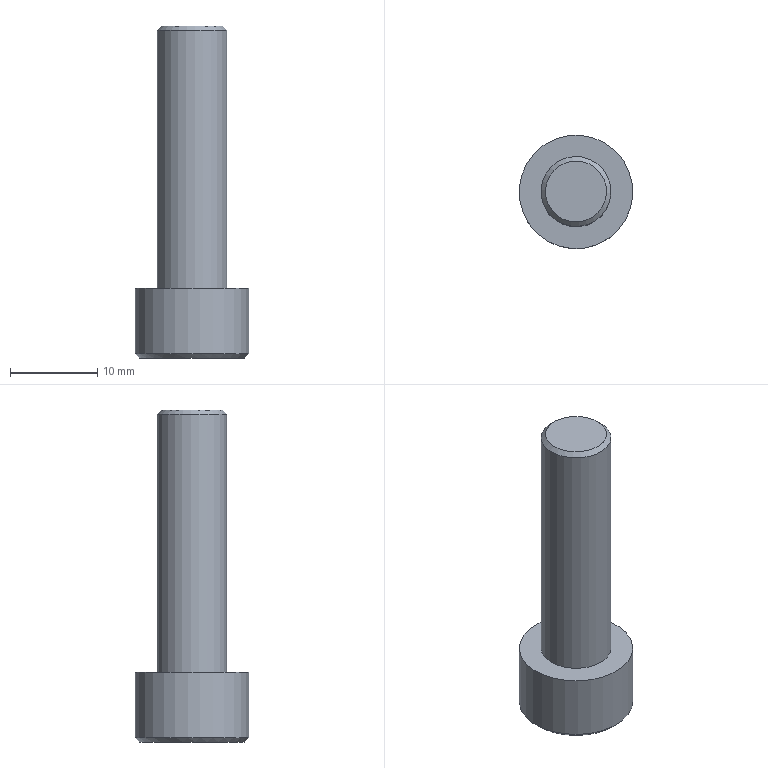Part | NX | features 18 2 | 1 solid | 21 faces | box 13 x 13 x 38 mm | volume 2425 mm3 | plane 15 | cone 4 | cylinder 2 | commonest cylinder face diameters 8 x1 13 x1
STEP:
#1=CARTESIAN_POINT('',(-32.713,-406.,-49.5));
#2=VERTEX_POINT('',#1);
#3=CARTESIAN_POINT('',(-29.713,-407.732,-50.5));
#4=VERTEX_POINT('',#3);
#5=CARTESIAN_POINT('',(-31.213,-406.866,-50.));
#6=DIRECTION('',(0.8321,-0.4804,-0.2774));
#7=VECTOR('',#6,1000.);
#8=LINE('',#5,#7);
#9=EDGE_CURVE('',#2,#4,#8,.T.);
#10=ORIENTED_EDGE('',*,*,#9,.F.);
#11=CARTESIAN_POINT('',(-35.713,-404.268,-50.5));
#12=VERTEX_POINT('',#11);
#13=CARTESIAN_POINT('',(-34.213,-405.134,-50.));
#14=DIRECTION('',(0.8321,-0.4804,0.2774));
#15=VECTOR('',#14,1000.);
#16=LINE('',#13,#15);
#17=EDGE_CURVE('',#12,#2,#16,.T.);
#18=ORIENTED_EDGE('',*,*,#17,.F.);
#19=CARTESIAN_POINT('',(-34.445,-403.,-50.5));
#20=VERTEX_POINT('',#19);
#21=CARTESIAN_POINT('',(-32.713,-406.,-50.5));
#22=DIRECTION('',(0.,0.,1.));
#23=DIRECTION('',(-0.866,0.5,0.));
#24=AXIS2_PLACEMENT_3D('',#21,#22,#23);
#25=CIRCLE('',#24,3.464);
#26=EDGE_CURVE('',#20,#12,#25,.T.);
#27=ORIENTED_EDGE('',*,*,#26,.F.);
#28=CARTESIAN_POINT('',(-30.981,-403.,-50.5));
#29=VERTEX_POINT('',#28);
#30=CARTESIAN_POINT('',(-32.713,-406.,-50.5));
#31=DIRECTION('',(0.,0.,1.));
#32=DIRECTION('',(-0.866,0.5,0.));
#33=AXIS2_PLACEMENT_3D('',#30,#31,#32);
#34=CIRCLE('',#33,3.464);
#35=EDGE_CURVE('',#29,#20,#34,.T.);
#36=ORIENTED_EDGE('',*,*,#35,.F.);
#37=CARTESIAN_POINT('',(-29.249,-406.,-50.5));
#38=VERTEX_POINT('',#37);
#39=CARTESIAN_POINT('',(-32.713,-406.,-50.5));
#40=DIRECTION('',(0.,0.,1.));
#41=DIRECTION('',(-0.866,0.5,0.));
#42=AXIS2_PLACEMENT_3D('',#39,#40,#41);
#43=CIRCLE('',#42,3.464);
#44=EDGE_CURVE('',#38,#29,#43,.T.);
#45=ORIENTED_EDGE('',*,*,#44,.F.);
#46=CARTESIAN_POINT('',(-32.713,-406.,-50.5));
#47=DIRECTION('',(0.,0.,1.));
#48=DIRECTION('',(-0.866,0.5,0.));
#49=AXIS2_PLACEMENT_3D('',#46,#47,#48);
#50=CIRCLE('',#49,3.464);
#51=EDGE_CURVE('',#4,#38,#50,.T.);
#52=ORIENTED_EDGE('',*,*,#51,.F.);
#53=EDGE_LOOP('',(#10,#18,#27,#36,#45,#52));
#54=FACE_BOUND('',#53,.T.);
#55=CARTESIAN_POINT('',(-32.713,-406.,-50.));
#56=DIRECTION('',(0.,0.,-1.));
#57=DIRECTION('',(-0.866,0.5,0.));
#58=AXIS2_PLACEMENT_3D('',#55,#56,#57);
#59=CONICAL_SURFACE('',#58,1.732,1.29);
#60=ADVANCED_FACE('',(#54),#59,.F.);
#61=CARTESIAN_POINT('',(-29.249,-408.,-17.));
#62=VERTEX_POINT('',#61);
#63=CARTESIAN_POINT('',(-32.713,-406.,-17.));
#64=DIRECTION('',(0.,0.,-1.));
#65=DIRECTION('',(0.866,-0.5,0.));
#66=AXIS2_PLACEMENT_3D('',#63,#64,#65);
#67=CIRCLE('',#66,4.);
#68=EDGE_CURVE('',#62,#62,#67,.T.);
#69=ORIENTED_EDGE('',*,*,#68,.F.);
#70=EDGE_LOOP('',(#69));
#71=FACE_BOUND('',#70,.T.);
#72=CARTESIAN_POINT('',(-29.682,-407.75,-16.5));
#73=VERTEX_POINT('',#72);
#74=CARTESIAN_POINT('',(-32.713,-406.,-16.5));
#75=DIRECTION('',(0.,0.,1.));
#76=DIRECTION('',(0.866,-0.5,0.));
#77=AXIS2_PLACEMENT_3D('',#74,#75,#76);
#78=CIRCLE('',#77,3.5);
#79=EDGE_CURVE('',#73,#73,#78,.T.);
#80=ORIENTED_EDGE('',*,*,#79,.F.);
#81=EDGE_LOOP('',(#80));
#82=FACE_BOUND('',#81,.T.);
#83=CARTESIAN_POINT('',(-32.713,-406.,-16.5));
#84=DIRECTION('',(0.,0.,-1.));
#85=DIRECTION('',(0.866,-0.5,0.));
#86=AXIS2_PLACEMENT_3D('',#83,#84,#85);
#87=CONICAL_SURFACE('',#86,3.5,0.7854);
#88=ADVANCED_FACE('',(#71,#82),#87,.T.);
#89=ORIENTED_EDGE('',*,*,#68,.T.);
#90=EDGE_LOOP('',(#89));
#91=FACE_BOUND('',#90,.T.);
#92=CARTESIAN_POINT('',(-36.177,-404.,-46.5));
#93=VERTEX_POINT('',#92);
#94=CARTESIAN_POINT('',(-32.713,-406.,-46.5));
#95=DIRECTION('',(0.,0.,1.));
#96=DIRECTION('',(-0.866,0.5,0.));
#97=AXIS2_PLACEMENT_3D('',#94,#95,#96);
#98=CIRCLE('',#97,4.);
#99=EDGE_CURVE('',#93,#93,#98,.T.);
#100=ORIENTED_EDGE('',*,*,#99,.T.);
#101=EDGE_LOOP('',(#100));
#102=FACE_BOUND('',#101,.T.);
#103=CARTESIAN_POINT('',(-32.713,-406.,-31.5));
#104=DIRECTION('',(0.,0.,1.));
#105=DIRECTION('',(-0.866,0.5,0.));
#106=AXIS2_PLACEMENT_3D('',#103,#104,#105);
#107=CYLINDRICAL_SURFACE('',#106,4.);
#108=ADVANCED_FACE('',(#91,#102),#107,.T.);
#109=ORIENTED_EDGE('',*,*,#79,.T.);
#110=EDGE_LOOP('',(#109));
#111=FACE_BOUND('',#110,.T.);
#112=CARTESIAN_POINT('',(-32.713,-406.,-16.5));
#113=DIRECTION('',(0.,0.,1.));
#114=DIRECTION('',(-0.866,0.5,0.));
#115=AXIS2_PLACEMENT_3D('',#112,#113,#114);
#116=PLANE('',#115);
#117=ADVANCED_FACE('',(#111),#116,.T.);
#118=CARTESIAN_POINT('',(-27.084,-409.25,-54.));
#119=VERTEX_POINT('',#118);
#120=CARTESIAN_POINT('',(-32.713,-406.,-54.));
#121=DIRECTION('',(0.,0.,1.));
#122=DIRECTION('',(0.866,-0.5,0.));
#123=AXIS2_PLACEMENT_3D('',#120,#121,#122);
#124=CIRCLE('',#123,6.5);
#125=EDGE_CURVE('',#119,#119,#124,.T.);
#126=ORIENTED_EDGE('',*,*,#125,.F.);
#127=EDGE_LOOP('',(#126));
#128=FACE_BOUND('',#127,.T.);
#129=CARTESIAN_POINT('',(-27.517,-409.,-54.5));
#130=VERTEX_POINT('',#129);
#131=CARTESIAN_POINT('',(-32.713,-406.,-54.5));
#132=DIRECTION('',(0.,0.,-1.));
#133=DIRECTION('',(0.866,-0.5,0.));
#134=AXIS2_PLACEMENT_3D('',#131,#132,#133);
#135=CIRCLE('',#134,6.);
#136=EDGE_CURVE('',#130,#130,#135,.T.);
#137=ORIENTED_EDGE('',*,*,#136,.F.);
#138=EDGE_LOOP('',(#137));
#139=FACE_BOUND('',#138,.T.);
#140=CARTESIAN_POINT('',(-32.713,-406.,-54.5));
#141=DIRECTION('',(0.,0.,1.));
#142=DIRECTION('',(0.866,-0.5,0.));
#143=AXIS2_PLACEMENT_3D('',#140,#141,#142);
#144=CONICAL_SURFACE('',#143,6.,0.7854);
#145=ADVANCED_FACE('',(#128,#139),#144,.T.);
#146=CARTESIAN_POINT('',(-38.342,-402.75,-46.5));
#147=VERTEX_POINT('',#146);
#148=CARTESIAN_POINT('',(-32.713,-406.,-46.5));
#149=DIRECTION('',(0.,0.,-1.));
#150=DIRECTION('',(-0.866,0.5,0.));
#151=AXIS2_PLACEMENT_3D('',#148,#149,#150);
#152=CIRCLE('',#151,6.5);
#153=EDGE_CURVE('',#147,#147,#152,.T.);
#154=ORIENTED_EDGE('',*,*,#153,.T.);
#155=EDGE_LOOP('',(#154));
#156=FACE_BOUND('',#155,.T.);
#157=ORIENTED_EDGE('',*,*,#125,.T.);
#158=EDGE_LOOP('',(#157));
#159=FACE_BOUND('',#158,.T.);
#160=CARTESIAN_POINT('',(-32.713,-406.,-50.5));
#161=DIRECTION('',(0.,0.,1.));
#162=DIRECTION('',(-0.866,0.5,0.));
#163=AXIS2_PLACEMENT_3D('',#160,#161,#162);
#164=CYLINDRICAL_SURFACE('',#163,6.5);
#165=ADVANCED_FACE('',(#156,#159),#164,.T.);
#166=CARTESIAN_POINT('',(-34.445,-403.,-54.5));
#167=VERTEX_POINT('',#166);
#168=CARTESIAN_POINT('',(-30.981,-403.,-54.5));
#169=VERTEX_POINT('',#168);
#170=CARTESIAN_POINT('',(-32.713,-403.,-54.5));
#171=DIRECTION('',(1.,0.,0.));
#172=VECTOR('',#171,1000.);
#173=LINE('',#170,#172);
#174=EDGE_CURVE('',#167,#169,#173,.T.);
#175=ORIENTED_EDGE('',*,*,#174,.F.);
#176=CARTESIAN_POINT('',(-36.177,-406.,-54.5));
#177=VERTEX_POINT('',#176);
#178=CARTESIAN_POINT('',(-35.311,-404.5,-54.5));
#179=DIRECTION('',(0.5,0.866,0.));
#180=VECTOR('',#179,1000.);
#181=LINE('',#178,#180);
#182=EDGE_CURVE('',#177,#167,#181,.T.);
#183=ORIENTED_EDGE('',*,*,#182,.F.);
#184=CARTESIAN_POINT('',(-34.445,-409.,-54.5));
#185=VERTEX_POINT('',#184);
#186=CARTESIAN_POINT('',(-35.311,-407.5,-54.5));
#187=DIRECTION('',(-0.5,0.866,0.));
#188=VECTOR('',#187,1000.);
#189=LINE('',#186,#188);
#190=EDGE_CURVE('',#185,#177,#189,.T.);
#191=ORIENTED_EDGE('',*,*,#190,.F.);
#192=CARTESIAN_POINT('',(-30.981,-409.,-54.5));
#193=VERTEX_POINT('',#192);
#194=CARTESIAN_POINT('',(-32.713,-409.,-54.5));
#195=DIRECTION('',(-1.,0.,0.));
#196=VECTOR('',#195,1000.);
#197=LINE('',#194,#196);
#198=EDGE_CURVE('',#193,#185,#197,.T.);
#199=ORIENTED_EDGE('',*,*,#198,.F.);
#200=CARTESIAN_POINT('',(-29.249,-406.,-54.5));
#201=VERTEX_POINT('',#200);
#202=CARTESIAN_POINT('',(-30.115,-407.5,-54.5));
#203=DIRECTION('',(-0.5,-0.866,0.));
#204=VECTOR('',#203,1000.);
#205=LINE('',#202,#204);
#206=EDGE_CURVE('',#201,#193,#205,.T.);
#207=ORIENTED_EDGE('',*,*,#206,.F.);
#208=CARTESIAN_POINT('',(-30.115,-404.5,-54.5));
#209=DIRECTION('',(0.5,-0.866,0.));
#210=VECTOR('',#209,1000.);
#211=LINE('',#208,#210);
#212=EDGE_CURVE('',#169,#201,#211,.T.);
#213=ORIENTED_EDGE('',*,*,#212,.F.);
#214=EDGE_LOOP('',(#175,#183,#191,#199,#207,#213));
#215=FACE_BOUND('',#214,.T.);
#216=ORIENTED_EDGE('',*,*,#136,.T.);
#217=EDGE_LOOP('',(#216));
#218=FACE_BOUND('',#217,.T.);
#219=CARTESIAN_POINT('',(-32.713,-406.,-54.5));
#220=DIRECTION('',(0.,0.,-1.));
#221=DIRECTION('',(0.866,-0.5,0.));
#222=AXIS2_PLACEMENT_3D('',#219,#220,#221);
#223=PLANE('',#222);
#224=ADVANCED_FACE('',(#215,#218),#223,.T.);
#225=CARTESIAN_POINT('',(-32.713,-403.,-50.5));
#226=DIRECTION('',(1.,0.,0.));
#227=VECTOR('',#226,1000.);
#228=LINE('',#225,#227);
#229=EDGE_CURVE('',#20,#29,#228,.T.);
#230=ORIENTED_EDGE('',*,*,#229,.T.);
#231=ORIENTED_EDGE('',*,*,#35,.T.);
#232=EDGE_LOOP('',(#230,#231));
#233=FACE_BOUND('',#232,.T.);
#234=CARTESIAN_POINT('',(-32.713,-406.,-50.5));
#235=DIRECTION('',(0.,0.,-1.));
#236=DIRECTION('',(0.866,-0.5,0.));
#237=AXIS2_PLACEMENT_3D('',#234,#235,#236);
#238=PLANE('',#237);
#239=ADVANCED_FACE('',(#233),#238,.F.);
#240=CARTESIAN_POINT('',(-36.177,-406.,-50.5));
#241=VERTEX_POINT('',#240);
#242=CARTESIAN_POINT('',(-35.311,-404.5,-50.5));
#243=DIRECTION('',(0.5,0.866,0.));
#244=VECTOR('',#243,1000.);
#245=LINE('',#242,#244);
#246=EDGE_CURVE('',#241,#20,#245,.T.);
#247=ORIENTED_EDGE('',*,*,#246,.T.);
#248=ORIENTED_EDGE('',*,*,#26,.T.);
#249=CARTESIAN_POINT('',(-32.713,-406.,-50.5));
#250=DIRECTION('',(0.,0.,1.));
#251=DIRECTION('',(-0.866,0.5,0.));
#252=AXIS2_PLACEMENT_3D('',#249,#250,#251);
#253=CIRCLE('',#252,3.464);
#254=EDGE_CURVE('',#12,#241,#253,.T.);
#255=ORIENTED_EDGE('',*,*,#254,.T.);
#256=EDGE_LOOP('',(#247,#248,#255));
#257=FACE_BOUND('',#256,.T.);
#258=CARTESIAN_POINT('',(-32.713,-406.,-50.5));
#259=DIRECTION('',(0.,0.,-1.));
#260=DIRECTION('',(0.866,-0.5,0.));
#261=AXIS2_PLACEMENT_3D('',#258,#259,#260);
#262=PLANE('',#261);
#263=ADVANCED_FACE('',(#257),#262,.F.);
#264=CARTESIAN_POINT('',(-34.445,-409.,-50.5));
#265=VERTEX_POINT('',#264);
#266=CARTESIAN_POINT('',(-35.311,-407.5,-50.5));
#267=DIRECTION('',(-0.5,0.866,0.));
#268=VECTOR('',#267,1000.);
#269=LINE('',#266,#268);
#270=EDGE_CURVE('',#265,#241,#269,.T.);
#271=ORIENTED_EDGE('',*,*,#270,.T.);
#272=CARTESIAN_POINT('',(-32.713,-406.,-50.5));
#273=DIRECTION('',(0.,0.,1.));
#274=DIRECTION('',(-0.866,0.5,0.));
#275=AXIS2_PLACEMENT_3D('',#272,#273,#274);
#276=CIRCLE('',#275,3.464);
#277=EDGE_CURVE('',#241,#265,#276,.T.);
#278=ORIENTED_EDGE('',*,*,#277,.T.);
#279=EDGE_LOOP('',(#271,#278));
#280=FACE_BOUND('',#279,.T.);
#281=CARTESIAN_POINT('',(-32.713,-406.,-50.5));
#282=DIRECTION('',(0.,0.,-1.));
#283=DIRECTION('',(0.866,-0.5,0.));
#284=AXIS2_PLACEMENT_3D('',#281,#282,#283);
#285=PLANE('',#284);
#286=ADVANCED_FACE('',(#280),#285,.F.);
#287=CARTESIAN_POINT('',(-30.981,-409.,-50.5));
#288=VERTEX_POINT('',#287);
#289=CARTESIAN_POINT('',(-32.713,-409.,-50.5));
#290=DIRECTION('',(-1.,0.,0.));
#291=VECTOR('',#290,1000.);
#292=LINE('',#289,#291);
#293=EDGE_CURVE('',#288,#265,#292,.T.);
#294=ORIENTED_EDGE('',*,*,#293,.T.);
#295=CARTESIAN_POINT('',(-32.713,-406.,-50.5));
#296=DIRECTION('',(0.,0.,1.));
#297=DIRECTION('',(-0.866,0.5,0.));
#298=AXIS2_PLACEMENT_3D('',#295,#296,#297);
#299=CIRCLE('',#298,3.464);
#300=EDGE_CURVE('',#265,#288,#299,.T.);
#301=ORIENTED_EDGE('',*,*,#300,.T.);
#302=EDGE_LOOP('',(#294,#301));
#303=FACE_BOUND('',#302,.T.);
#304=CARTESIAN_POINT('',(-32.713,-406.,-50.5));
#305=DIRECTION('',(0.,0.,-1.));
#306=DIRECTION('',(0.866,-0.5,0.));
#307=AXIS2_PLACEMENT_3D('',#304,#305,#306);
#308=PLANE('',#307);
#309=ADVANCED_FACE('',(#303),#308,.F.);
#310=CARTESIAN_POINT('',(-30.115,-407.5,-50.5));
#311=DIRECTION('',(-0.5,-0.866,0.));
#312=VECTOR('',#311,1000.);
#313=LINE('',#310,#312);
#314=EDGE_CURVE('',#38,#288,#313,.T.);
#315=ORIENTED_EDGE('',*,*,#314,.T.);
#316=CARTESIAN_POINT('',(-32.713,-406.,-50.5));
#317=DIRECTION('',(0.,0.,1.));
#318=DIRECTION('',(-0.866,0.5,0.));
#319=AXIS2_PLACEMENT_3D('',#316,#317,#318);
#320=CIRCLE('',#319,3.464);
#321=EDGE_CURVE('',#288,#4,#320,.T.);
#322=ORIENTED_EDGE('',*,*,#321,.T.);
#323=ORIENTED_EDGE('',*,*,#51,.T.);
#324=EDGE_LOOP('',(#315,#322,#323));
#325=FACE_BOUND('',#324,.T.);
#326=CARTESIAN_POINT('',(-32.713,-406.,-50.5));
#327=DIRECTION('',(0.,0.,-1.));
#328=DIRECTION('',(0.866,-0.5,0.));
#329=AXIS2_PLACEMENT_3D('',#326,#327,#328);
#330=PLANE('',#329);
#331=ADVANCED_FACE('',(#325),#330,.F.);
#332=CARTESIAN_POINT('',(-30.115,-404.5,-50.5));
#333=DIRECTION('',(0.5,-0.866,0.));
#334=VECTOR('',#333,1000.);
#335=LINE('',#332,#334);
#336=EDGE_CURVE('',#29,#38,#335,.T.);
#337=ORIENTED_EDGE('',*,*,#336,.T.);
#338=ORIENTED_EDGE('',*,*,#44,.T.);
#339=EDGE_LOOP('',(#337,#338));
#340=FACE_BOUND('',#339,.T.);
#341=CARTESIAN_POINT('',(-32.713,-406.,-50.5));
#342=DIRECTION('',(0.,0.,-1.));
#343=DIRECTION('',(0.866,-0.5,0.));
#344=AXIS2_PLACEMENT_3D('',#341,#342,#343);
#345=PLANE('',#344);
#346=ADVANCED_FACE('',(#340),#345,.F.);
#347=ORIENTED_EDGE('',*,*,#9,.T.);
#348=ORIENTED_EDGE('',*,*,#321,.F.);
#349=ORIENTED_EDGE('',*,*,#300,.F.);
#350=ORIENTED_EDGE('',*,*,#277,.F.);
#351=ORIENTED_EDGE('',*,*,#254,.F.);
#352=ORIENTED_EDGE('',*,*,#17,.T.);
#353=EDGE_LOOP('',(#347,#348,#349,#350,#351,#352));
#354=FACE_BOUND('',#353,.T.);
#355=CARTESIAN_POINT('',(-32.713,-406.,-50.));
#356=DIRECTION('',(0.,0.,-1.));
#357=DIRECTION('',(-0.866,0.5,0.));
#358=AXIS2_PLACEMENT_3D('',#355,#356,#357);
#359=CONICAL_SURFACE('',#358,1.732,1.29);
#360=ADVANCED_FACE('',(#354),#359,.F.);
#361=CARTESIAN_POINT('',(-30.981,-403.,-52.5));
#362=DIRECTION('',(0.,0.,1.));
#363=VECTOR('',#362,1000.);
#364=LINE('',#361,#363);
#365=EDGE_CURVE('',#169,#29,#364,.T.);
#366=ORIENTED_EDGE('',*,*,#365,.T.);
#367=ORIENTED_EDGE('',*,*,#229,.F.);
#368=CARTESIAN_POINT('',(-34.445,-403.,-52.5));
#369=DIRECTION('',(0.,0.,1.));
#370=VECTOR('',#369,1000.);
#371=LINE('',#368,#370);
#372=EDGE_CURVE('',#167,#20,#371,.T.);
#373=ORIENTED_EDGE('',*,*,#372,.F.);
#374=ORIENTED_EDGE('',*,*,#174,.T.);
#375=EDGE_LOOP('',(#366,#367,#373,#374));
#376=FACE_BOUND('',#375,.T.);
#377=CARTESIAN_POINT('',(-32.713,-403.,-52.5));
#378=DIRECTION('',(0.,-1.,0.));
#379=DIRECTION('',(0.,0.,1.));
#380=AXIS2_PLACEMENT_3D('',#377,#378,#379);
#381=PLANE('',#380);
#382=ADVANCED_FACE('',(#376),#381,.T.);
#383=CARTESIAN_POINT('',(-29.249,-406.,-52.5));
#384=DIRECTION('',(0.,0.,1.));
#385=VECTOR('',#384,1000.);
#386=LINE('',#383,#385);
#387=EDGE_CURVE('',#201,#38,#386,.T.);
#388=ORIENTED_EDGE('',*,*,#387,.T.);
#389=ORIENTED_EDGE('',*,*,#336,.F.);
#390=ORIENTED_EDGE('',*,*,#365,.F.);
#391=ORIENTED_EDGE('',*,*,#212,.T.);
#392=EDGE_LOOP('',(#388,#389,#390,#391));
#393=FACE_BOUND('',#392,.T.);
#394=CARTESIAN_POINT('',(-30.115,-404.5,-52.5));
#395=DIRECTION('',(-0.866,-0.5,0.));
#396=DIRECTION('',(0.,0.,-1.));
#397=AXIS2_PLACEMENT_3D('',#394,#395,#396);
#398=PLANE('',#397);
#399=ADVANCED_FACE('',(#393),#398,.T.);
#400=CARTESIAN_POINT('',(-30.981,-409.,-52.5));
#401=DIRECTION('',(0.,0.,1.));
#402=VECTOR('',#401,1000.);
#403=LINE('',#400,#402);
#404=EDGE_CURVE('',#193,#288,#403,.T.);
#405=ORIENTED_EDGE('',*,*,#404,.T.);
#406=ORIENTED_EDGE('',*,*,#314,.F.);
#407=ORIENTED_EDGE('',*,*,#387,.F.);
#408=ORIENTED_EDGE('',*,*,#206,.T.);
#409=EDGE_LOOP('',(#405,#406,#407,#408));
#410=FACE_BOUND('',#409,.T.);
#411=CARTESIAN_POINT('',(-30.115,-407.5,-52.5));
#412=DIRECTION('',(-0.866,0.5,0.));
#413=DIRECTION('',(0.,0.,-1.));
#414=AXIS2_PLACEMENT_3D('',#411,#412,#413);
#415=PLANE('',#414);
#416=ADVANCED_FACE('',(#410),#415,.T.);
#417=CARTESIAN_POINT('',(-34.445,-409.,-52.5));
#418=DIRECTION('',(0.,0.,1.));
#419=VECTOR('',#418,1000.);
#420=LINE('',#417,#419);
#421=EDGE_CURVE('',#185,#265,#420,.T.);
#422=ORIENTED_EDGE('',*,*,#421,.T.);
#423=ORIENTED_EDGE('',*,*,#293,.F.);
#424=ORIENTED_EDGE('',*,*,#404,.F.);
#425=ORIENTED_EDGE('',*,*,#198,.T.);
#426=EDGE_LOOP('',(#422,#423,#424,#425));
#427=FACE_BOUND('',#426,.T.);
#428=CARTESIAN_POINT('',(-32.713,-409.,-52.5));
#429=DIRECTION('',(0.,1.,0.));
#430=DIRECTION('',(0.,0.,-1.));
#431=AXIS2_PLACEMENT_3D('',#428,#429,#430);
#432=PLANE('',#431);
#433=ADVANCED_FACE('',(#427),#432,.T.);
#434=CARTESIAN_POINT('',(-36.177,-406.,-52.5));
#435=DIRECTION('',(0.,0.,1.));
#436=VECTOR('',#435,1000.);
#437=LINE('',#434,#436);
#438=EDGE_CURVE('',#177,#241,#437,.T.);
#439=ORIENTED_EDGE('',*,*,#438,.T.);
#440=ORIENTED_EDGE('',*,*,#270,.F.);
#441=ORIENTED_EDGE('',*,*,#421,.F.);
#442=ORIENTED_EDGE('',*,*,#190,.T.);
#443=EDGE_LOOP('',(#439,#440,#441,#442));
#444=FACE_BOUND('',#443,.T.);
#445=CARTESIAN_POINT('',(-35.311,-407.5,-52.5));
#446=DIRECTION('',(0.866,0.5,0.));
#447=DIRECTION('',(0.,0.,1.));
#448=AXIS2_PLACEMENT_3D('',#445,#446,#447);
#449=PLANE('',#448);
#450=ADVANCED_FACE('',(#444),#449,.T.);
#451=ORIENTED_EDGE('',*,*,#372,.T.);
#452=ORIENTED_EDGE('',*,*,#246,.F.);
#453=ORIENTED_EDGE('',*,*,#438,.F.);
#454=ORIENTED_EDGE('',*,*,#182,.T.);
#455=EDGE_LOOP('',(#451,#452,#453,#454));
#456=FACE_BOUND('',#455,.T.);
#457=CARTESIAN_POINT('',(-35.311,-404.5,-52.5));
#458=DIRECTION('',(0.866,-0.5,0.));
#459=DIRECTION('',(0.,0.,1.));
#460=AXIS2_PLACEMENT_3D('',#457,#458,#459);
#461=PLANE('',#460);
#462=ADVANCED_FACE('',(#456),#461,.T.);
#463=ORIENTED_EDGE('',*,*,#99,.F.);
#464=EDGE_LOOP('',(#463));
#465=FACE_BOUND('',#464,.T.);
#466=ORIENTED_EDGE('',*,*,#153,.F.);
#467=EDGE_LOOP('',(#466));
#468=FACE_BOUND('',#467,.T.);
#469=CARTESIAN_POINT('',(-32.713,-406.,-46.5));
#470=DIRECTION('',(0.,0.,1.));
#471=DIRECTION('',(-0.866,0.5,0.));
#472=AXIS2_PLACEMENT_3D('',#469,#470,#471);
#473=PLANE('',#472);
#474=ADVANCED_FACE('',(#465,#468),#473,.T.);
#475=CLOSED_SHELL('',(#60,#88,#108,#117,#145,#165,#224,#239,#263,#286,#309,#331,#346,#360,#382,#399,#416,#433,#450,#462,#474));
#476=MANIFOLD_SOLID_BREP('',#475);
#477=(LENGTH_UNIT()NAMED_UNIT(*)SI_UNIT(.MILLI.,.METRE.));
#478=UNCERTAINTY_MEASURE_WITH_UNIT(LENGTH_MEASURE(0.00001),#477,'','');
#479=(NAMED_UNIT(*)PLANE_ANGLE_UNIT()SI_UNIT($,.RADIAN.));
#480=(NAMED_UNIT(*)SI_UNIT($,.STERADIAN.)SOLID_ANGLE_UNIT());
#481=(GEOMETRIC_REPRESENTATION_CONTEXT(3)GLOBAL_UNCERTAINTY_ASSIGNED_CONTEXT((#478))GLOBAL_UNIT_ASSIGNED_CONTEXT((#477,#479,#480))REPRESENTATION_CONTEXT('',''));
#482=ADVANCED_BREP_SHAPE_REPRESENTATION('',(#476),#481);